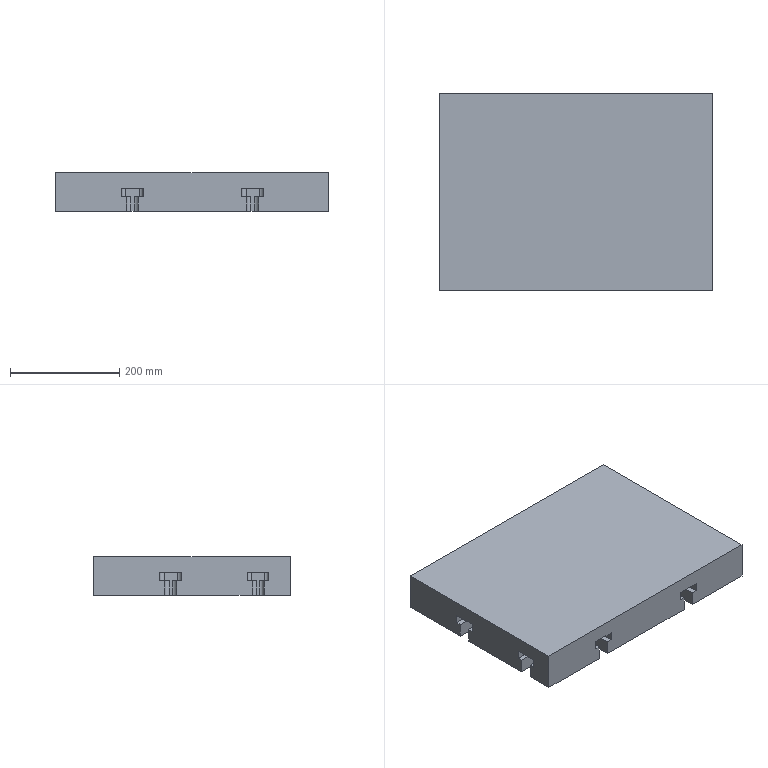Part | STEP file | 200 mesh_id2030 | 1 solid | 102 faces | box 500 x 360 x 70 mm | volume 11688110 mm3 | plane 70 | cylinder 32 | commonest cylinder face diameters 16 x32